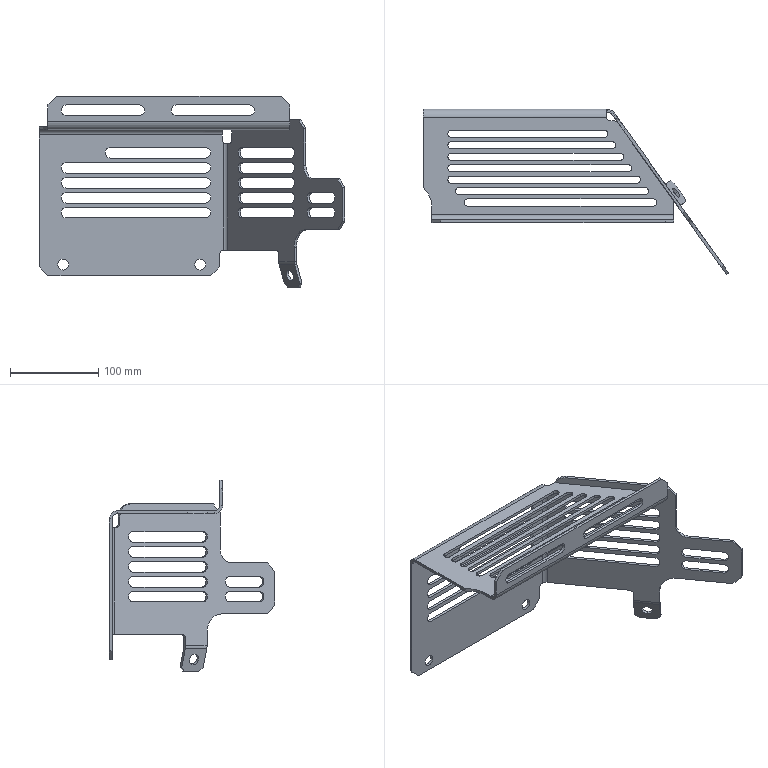Part | SolidWorks | features SM3dBend 4, FlatPattern 1, SMBaseFlange 1, SheetMetal 1 | 1 solid | 163 faces | box 347.398 x 187.972 x 217.987 mm | volume 228899 mm3 | plane 94 | cylinder 66 | spline 3 | commonest cylinder face diameters 12 x33 8 x14 12.5 x6 10 x5 18.4 x4 30 x2